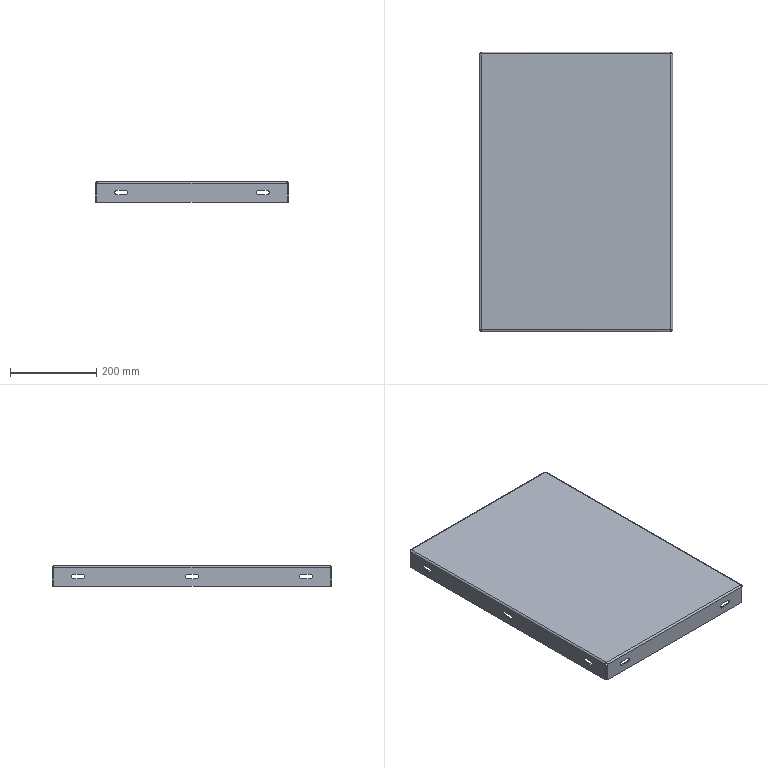Part | NX | features BREP 1 | 1 solid | 78 faces | box 449 x 649 x 48 mm | volume 1150610 mm3 | plane 42 | cylinder 28 | spline 8 | commonest cylinder face diameters 10.5 x20 2 x4 8 x4